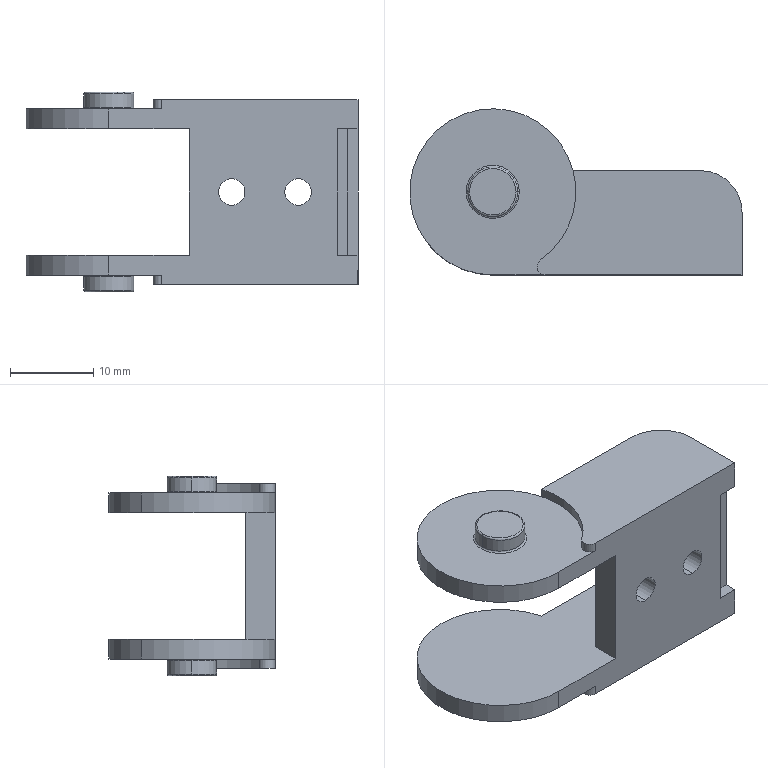Part | STEP file | TWD15-C15-R28-3_fix | 1 solid | 50 faces | box 40 x 20 x 24 mm | volume 4424 mm3 | plane 20 | cylinder 18 | torus 8 | cone 4 | commonest cylinder face diameters 20 x6 3.2 x4 6 x4 2 x2 10 x2
STEP:
#1=CARTESIAN_POINT('',(-15.2,2.5,-1.6));
#2=VERTEX_POINT('',#1);
#3=CARTESIAN_POINT('',(-15.2,2.5,1.6));
#4=VERTEX_POINT('',#3);
#5=CARTESIAN_POINT('',(-15.2,2.5,0.));
#6=DIRECTION('',(0.,-1.,0.));
#7=DIRECTION('',(0.,0.,1.));
#8=AXIS2_PLACEMENT_3D('',#5,#6,#7);
#9=CIRCLE('',#8,1.6);
#10=EDGE_CURVE('',#2,#4,#9,.T.);
#11=ORIENTED_EDGE('',*,*,#10,.F.);
#12=CARTESIAN_POINT('',(-15.2,0.,-1.6));
#13=VERTEX_POINT('',#12);
#14=CARTESIAN_POINT('',(-15.2,0.,-1.6));
#15=DIRECTION('',(0.,-1.,0.));
#16=VECTOR('',#15,1000.);
#17=LINE('',#14,#16);
#18=EDGE_CURVE('',#2,#13,#17,.T.);
#19=ORIENTED_EDGE('',*,*,#18,.T.);
#20=CARTESIAN_POINT('',(-15.2,0.,1.6));
#21=VERTEX_POINT('',#20);
#22=CARTESIAN_POINT('',(-15.2,0.,0.));
#23=DIRECTION('',(0.,-1.,0.));
#24=DIRECTION('',(0.,0.,-1.));
#25=AXIS2_PLACEMENT_3D('',#22,#23,#24);
#26=CIRCLE('',#25,1.6);
#27=EDGE_CURVE('',#13,#21,#26,.T.);
#28=ORIENTED_EDGE('',*,*,#27,.T.);
#29=CARTESIAN_POINT('',(-15.2,0.,1.6));
#30=DIRECTION('',(0.,-1.,0.));
#31=VECTOR('',#30,1000.);
#32=LINE('',#29,#31);
#33=EDGE_CURVE('',#4,#21,#32,.T.);
#34=ORIENTED_EDGE('',*,*,#33,.F.);
#35=EDGE_LOOP('',(#11,#19,#28,#34));
#36=FACE_OUTER_BOUND('',#35,.T.);
#37=CARTESIAN_POINT('',(-15.2,0.,0.));
#38=DIRECTION('',(0.,-1.,0.));
#39=DIRECTION('',(0.000000142,0.,1.));
#40=AXIS2_PLACEMENT_3D('',#37,#38,#39);
#41=CYLINDRICAL_SURFACE('',#40,1.6);
#42=ADVANCED_FACE('',(#36),#41,.F.);
#43=ORIENTED_EDGE('',*,*,#10,.T.);
#44=CARTESIAN_POINT('',(-15.2,3.5,2.6));
#45=VERTEX_POINT('',#44);
#46=CARTESIAN_POINT('',(-15.2,3.5,2.6));
#47=DIRECTION('',(0.,0.7071,0.7071));
#48=VECTOR('',#47,1000.);
#49=LINE('',#46,#48);
#50=EDGE_CURVE('',#4,#45,#49,.T.);
#51=ORIENTED_EDGE('',*,*,#50,.T.);
#52=CARTESIAN_POINT('',(-15.2,3.5,-2.6));
#53=VERTEX_POINT('',#52);
#54=CARTESIAN_POINT('',(-15.2,3.5,0.));
#55=DIRECTION('',(0.,-1.,0.));
#56=DIRECTION('',(0.,0.,1.));
#57=AXIS2_PLACEMENT_3D('',#54,#55,#56);
#58=CIRCLE('',#57,2.6);
#59=EDGE_CURVE('',#53,#45,#58,.T.);
#60=ORIENTED_EDGE('',*,*,#59,.F.);
#61=CARTESIAN_POINT('',(-15.2,3.5,-2.6));
#62=DIRECTION('',(0.,0.7071,-0.7071));
#63=VECTOR('',#62,1000.);
#64=LINE('',#61,#63);
#65=EDGE_CURVE('',#2,#53,#64,.T.);
#66=ORIENTED_EDGE('',*,*,#65,.F.);
#67=EDGE_LOOP('',(#43,#51,#60,#66));
#68=FACE_OUTER_BOUND('',#67,.T.);
#69=CARTESIAN_POINT('',(-15.2,3.5,0.));
#70=DIRECTION('',(0.,1.,0.));
#71=DIRECTION('',(0.,0.,-1.));
#72=AXIS2_PLACEMENT_3D('',#69,#70,#71);
#73=CONICAL_SURFACE('',#72,2.6,0.7854);
#74=ADVANCED_FACE('',(#68),#73,.F.);
#75=CARTESIAN_POINT('',(-7.2,2.5,-1.6));
#76=VERTEX_POINT('',#75);
#77=CARTESIAN_POINT('',(-7.2,2.5,1.6));
#78=VERTEX_POINT('',#77);
#79=CARTESIAN_POINT('',(-7.2,2.5,0.));
#80=DIRECTION('',(0.,-1.,0.));
#81=DIRECTION('',(0.,0.,1.));
#82=AXIS2_PLACEMENT_3D('',#79,#80,#81);
#83=CIRCLE('',#82,1.6);
#84=EDGE_CURVE('',#76,#78,#83,.T.);
#85=ORIENTED_EDGE('',*,*,#84,.F.);
#86=CARTESIAN_POINT('',(-7.2,0.,-1.6));
#87=VERTEX_POINT('',#86);
#88=CARTESIAN_POINT('',(-7.2,0.,-1.6));
#89=DIRECTION('',(0.,-1.,0.));
#90=VECTOR('',#89,1000.);
#91=LINE('',#88,#90);
#92=EDGE_CURVE('',#76,#87,#91,.T.);
#93=ORIENTED_EDGE('',*,*,#92,.T.);
#94=CARTESIAN_POINT('',(-7.2,0.,1.6));
#95=VERTEX_POINT('',#94);
#96=CARTESIAN_POINT('',(-7.2,0.,0.));
#97=DIRECTION('',(0.,-1.,0.));
#98=DIRECTION('',(0.,0.,-1.));
#99=AXIS2_PLACEMENT_3D('',#96,#97,#98);
#100=CIRCLE('',#99,1.6);
#101=EDGE_CURVE('',#87,#95,#100,.T.);
#102=ORIENTED_EDGE('',*,*,#101,.T.);
#103=CARTESIAN_POINT('',(-7.2,0.,1.6));
#104=DIRECTION('',(0.,-1.,0.));
#105=VECTOR('',#104,1000.);
#106=LINE('',#103,#105);
#107=EDGE_CURVE('',#78,#95,#106,.T.);
#108=ORIENTED_EDGE('',*,*,#107,.F.);
#109=EDGE_LOOP('',(#85,#93,#102,#108));
#110=FACE_OUTER_BOUND('',#109,.T.);
#111=CARTESIAN_POINT('',(-7.2,0.,0.));
#112=DIRECTION('',(0.,-1.,0.));
#113=DIRECTION('',(0.000000142,0.,1.));
#114=AXIS2_PLACEMENT_3D('',#111,#112,#113);
#115=CYLINDRICAL_SURFACE('',#114,1.6);
#116=ADVANCED_FACE('',(#110),#115,.F.);
#117=ORIENTED_EDGE('',*,*,#84,.T.);
#118=CARTESIAN_POINT('',(-7.2,3.5,2.6));
#119=VERTEX_POINT('',#118);
#120=CARTESIAN_POINT('',(-7.2,3.5,2.6));
#121=DIRECTION('',(0.,0.7071,0.7071));
#122=VECTOR('',#121,1000.);
#123=LINE('',#120,#122);
#124=EDGE_CURVE('',#78,#119,#123,.T.);
#125=ORIENTED_EDGE('',*,*,#124,.T.);
#126=CARTESIAN_POINT('',(-7.2,3.5,-2.6));
#127=VERTEX_POINT('',#126);
#128=CARTESIAN_POINT('',(-7.2,3.5,0.));
#129=DIRECTION('',(0.,-1.,0.));
#130=DIRECTION('',(-0.000000142,0.,1.));
#131=AXIS2_PLACEMENT_3D('',#128,#129,#130);
#132=CIRCLE('',#131,2.6);
#133=EDGE_CURVE('',#127,#119,#132,.T.);
#134=ORIENTED_EDGE('',*,*,#133,.F.);
#135=CARTESIAN_POINT('',(-7.2,3.5,-2.6));
#136=DIRECTION('',(0.,0.7071,-0.7071));
#137=VECTOR('',#136,1000.);
#138=LINE('',#135,#137);
#139=EDGE_CURVE('',#76,#127,#138,.T.);
#140=ORIENTED_EDGE('',*,*,#139,.F.);
#141=EDGE_LOOP('',(#117,#125,#134,#140));
#142=FACE_OUTER_BOUND('',#141,.T.);
#143=CARTESIAN_POINT('',(-7.2,3.5,0.));
#144=DIRECTION('',(0.,1.,0.));
#145=DIRECTION('',(0.,0.,-1.));
#146=AXIS2_PLACEMENT_3D('',#143,#144,#145);
#147=CONICAL_SURFACE('',#146,2.6,0.7854);
#148=ADVANCED_FACE('',(#142),#147,.F.);
#149=CARTESIAN_POINT('',(-33.2,10.,10.));
#150=VERTEX_POINT('',#149);
#151=CARTESIAN_POINT('',(-26.8,10.,10.));
#152=VERTEX_POINT('',#151);
#153=CARTESIAN_POINT('',(-30.,10.,10.));
#154=DIRECTION('',(0.,0.,-1.));
#155=DIRECTION('',(1.,0.,0.));
#156=AXIS2_PLACEMENT_3D('',#153,#154,#155);
#157=CIRCLE('',#156,3.2);
#158=EDGE_CURVE('',#150,#152,#157,.T.);
#159=ORIENTED_EDGE('',*,*,#158,.F.);
#160=CARTESIAN_POINT('',(-33.,10.,10.2));
#161=VERTEX_POINT('',#160);
#162=CARTESIAN_POINT('',(-33.2,10.,10.2));
#163=DIRECTION('',(0.,-1.,0.));
#164=DIRECTION('',(1.,0.,0.));
#165=AXIS2_PLACEMENT_3D('',#162,#163,#164);
#166=CIRCLE('',#165,0.2);
#167=EDGE_CURVE('',#150,#161,#166,.T.);
#168=ORIENTED_EDGE('',*,*,#167,.T.);
#169=CARTESIAN_POINT('',(-27.,10.,10.2));
#170=VERTEX_POINT('',#169);
#171=CARTESIAN_POINT('',(-30.,10.,10.2));
#172=DIRECTION('',(0.,0.,-1.));
#173=DIRECTION('',(-1.,0.,0.));
#174=AXIS2_PLACEMENT_3D('',#171,#172,#173);
#175=CIRCLE('',#174,3.);
#176=EDGE_CURVE('',#161,#170,#175,.T.);
#177=ORIENTED_EDGE('',*,*,#176,.T.);
#178=CARTESIAN_POINT('',(-26.8,10.,10.2));
#179=DIRECTION('',(0.,1.,0.));
#180=DIRECTION('',(-1.,0.,0.));
#181=AXIS2_PLACEMENT_3D('',#178,#179,#180);
#182=CIRCLE('',#181,0.2);
#183=EDGE_CURVE('',#152,#170,#182,.T.);
#184=ORIENTED_EDGE('',*,*,#183,.F.);
#185=EDGE_LOOP('',(#159,#168,#177,#184));
#186=FACE_OUTER_BOUND('',#185,.T.);
#187=CARTESIAN_POINT('',(-30.,10.,10.2));
#188=DIRECTION('',(0.,0.,-1.));
#189=DIRECTION('',(1.,0.,0.));
#190=AXIS2_PLACEMENT_3D('',#187,#188,#189);
#191=TOROIDAL_SURFACE('',#190,3.2,0.2);
#192=ADVANCED_FACE('',(#186),#191,.F.);
#193=CARTESIAN_POINT('',(-27.,10.,11.8));
#194=VERTEX_POINT('',#193);
#195=CARTESIAN_POINT('',(-33.,10.,11.8));
#196=VERTEX_POINT('',#195);
#197=CARTESIAN_POINT('',(-30.,10.,11.8));
#198=DIRECTION('',(0.,0.,-1.));
#199=DIRECTION('',(-1.,0.,0.));
#200=AXIS2_PLACEMENT_3D('',#197,#198,#199);
#201=CIRCLE('',#200,3.);
#202=EDGE_CURVE('',#194,#196,#201,.T.);
#203=ORIENTED_EDGE('',*,*,#202,.T.);
#204=CARTESIAN_POINT('',(-33.,10.,10.));
#205=DIRECTION('',(0.,0.,-1.));
#206=VECTOR('',#205,1000.);
#207=LINE('',#204,#206);
#208=EDGE_CURVE('',#196,#161,#207,.T.);
#209=ORIENTED_EDGE('',*,*,#208,.T.);
#210=CARTESIAN_POINT('',(-30.,10.,10.2));
#211=DIRECTION('',(0.,0.,-1.));
#212=DIRECTION('',(-1.,0.,0.));
#213=AXIS2_PLACEMENT_3D('',#210,#211,#212);
#214=CIRCLE('',#213,3.);
#215=EDGE_CURVE('',#170,#161,#214,.T.);
#216=ORIENTED_EDGE('',*,*,#215,.F.);
#217=CARTESIAN_POINT('',(-27.,10.,10.));
#218=DIRECTION('',(0.,0.,-1.));
#219=VECTOR('',#218,1000.);
#220=LINE('',#217,#219);
#221=EDGE_CURVE('',#194,#170,#220,.T.);
#222=ORIENTED_EDGE('',*,*,#221,.F.);
#223=EDGE_LOOP('',(#203,#209,#216,#222));
#224=FACE_OUTER_BOUND('',#223,.T.);
#225=CARTESIAN_POINT('',(-30.,10.,10.));
#226=DIRECTION('',(0.,0.,-1.));
#227=DIRECTION('',(1.,0.000000001,0.));
#228=AXIS2_PLACEMENT_3D('',#225,#226,#227);
#229=CYLINDRICAL_SURFACE('',#228,3.);
#230=ADVANCED_FACE('',(#224),#229,.T.);
#231=CARTESIAN_POINT('',(-27.2,10.,12.));
#232=VERTEX_POINT('',#231);
#233=CARTESIAN_POINT('',(-32.8,10.,12.));
#234=VERTEX_POINT('',#233);
#235=CARTESIAN_POINT('',(-30.,10.,12.));
#236=DIRECTION('',(0.,0.,-1.));
#237=DIRECTION('',(-1.,0.,0.));
#238=AXIS2_PLACEMENT_3D('',#235,#236,#237);
#239=CIRCLE('',#238,2.8);
#240=EDGE_CURVE('',#232,#234,#239,.T.);
#241=ORIENTED_EDGE('',*,*,#240,.T.);
#242=CARTESIAN_POINT('',(-32.8,10.,11.8));
#243=DIRECTION('',(0.000000142,-1.,0.));
#244=DIRECTION('',(1.,0.000000142,0.));
#245=AXIS2_PLACEMENT_3D('',#242,#243,#244);
#246=CIRCLE('',#245,0.2);
#247=EDGE_CURVE('',#234,#196,#246,.T.);
#248=ORIENTED_EDGE('',*,*,#247,.T.);
#249=ORIENTED_EDGE('',*,*,#202,.F.);
#250=CARTESIAN_POINT('',(-27.2,10.,11.8));
#251=DIRECTION('',(-0.000000142,1.,0.));
#252=DIRECTION('',(-1.,-0.000000142,0.));
#253=AXIS2_PLACEMENT_3D('',#250,#251,#252);
#254=CIRCLE('',#253,0.2);
#255=EDGE_CURVE('',#232,#194,#254,.T.);
#256=ORIENTED_EDGE('',*,*,#255,.F.);
#257=EDGE_LOOP('',(#241,#248,#249,#256));
#258=FACE_OUTER_BOUND('',#257,.T.);
#259=CARTESIAN_POINT('',(-30.,10.,11.8));
#260=DIRECTION('',(0.,0.,-1.));
#261=DIRECTION('',(1.,0.000000142,0.));
#262=AXIS2_PLACEMENT_3D('',#259,#260,#261);
#263=TOROIDAL_SURFACE('',#262,2.8,0.2);
#264=ADVANCED_FACE('',(#258),#263,.T.);
#265=CARTESIAN_POINT('',(-27.,10.,-11.8));
#266=VERTEX_POINT('',#265);
#267=CARTESIAN_POINT('',(-33.,10.,-11.8));
#268=VERTEX_POINT('',#267);
#269=CARTESIAN_POINT('',(-30.,10.,-11.8));
#270=DIRECTION('',(0.,0.,-1.));
#271=DIRECTION('',(-1.,0.,0.));
#272=AXIS2_PLACEMENT_3D('',#269,#270,#271);
#273=CIRCLE('',#272,3.);
#274=EDGE_CURVE('',#266,#268,#273,.T.);
#275=ORIENTED_EDGE('',*,*,#274,.T.);
#276=CARTESIAN_POINT('',(-32.8,10.,-12.));
#277=VERTEX_POINT('',#276);
#278=CARTESIAN_POINT('',(-32.8,10.,-11.8));
#279=DIRECTION('',(0.,-1.,0.));
#280=DIRECTION('',(1.,0.,0.));
#281=AXIS2_PLACEMENT_3D('',#278,#279,#280);
#282=CIRCLE('',#281,0.2);
#283=EDGE_CURVE('',#268,#277,#282,.T.);
#284=ORIENTED_EDGE('',*,*,#283,.T.);
#285=CARTESIAN_POINT('',(-27.2,10.,-12.));
#286=VERTEX_POINT('',#285);
#287=CARTESIAN_POINT('',(-30.,10.,-12.));
#288=DIRECTION('',(0.,0.,-1.));
#289=DIRECTION('',(1.,-0.000000142,0.));
#290=AXIS2_PLACEMENT_3D('',#287,#288,#289);
#291=CIRCLE('',#290,2.8);
#292=EDGE_CURVE('',#286,#277,#291,.T.);
#293=ORIENTED_EDGE('',*,*,#292,.F.);
#294=CARTESIAN_POINT('',(-27.2,10.,-11.8));
#295=DIRECTION('',(0.,1.,0.));
#296=DIRECTION('',(-1.,0.,0.));
#297=AXIS2_PLACEMENT_3D('',#294,#295,#296);
#298=CIRCLE('',#297,0.2);
#299=EDGE_CURVE('',#266,#286,#298,.T.);
#300=ORIENTED_EDGE('',*,*,#299,.F.);
#301=EDGE_LOOP('',(#275,#284,#293,#300));
#302=FACE_OUTER_BOUND('',#301,.T.);
#303=CARTESIAN_POINT('',(-30.,10.,-11.8));
#304=DIRECTION('',(0.,0.,-1.));
#305=DIRECTION('',(1.,0.,0.));
#306=AXIS2_PLACEMENT_3D('',#303,#304,#305);
#307=TOROIDAL_SURFACE('',#306,2.8,0.2);
#308=ADVANCED_FACE('',(#302),#307,.T.);
#309=CARTESIAN_POINT('',(-27.,10.,-10.2));
#310=VERTEX_POINT('',#309);
#311=CARTESIAN_POINT('',(-33.,10.,-10.2));
#312=VERTEX_POINT('',#311);
#313=CARTESIAN_POINT('',(-30.,10.,-10.2));
#314=DIRECTION('',(0.,0.,-1.));
#315=DIRECTION('',(-1.,0.,0.));
#316=AXIS2_PLACEMENT_3D('',#313,#314,#315);
#317=CIRCLE('',#316,3.);
#318=EDGE_CURVE('',#310,#312,#317,.T.);
#319=ORIENTED_EDGE('',*,*,#318,.T.);
#320=CARTESIAN_POINT('',(-33.,10.,-12.));
#321=DIRECTION('',(0.,0.,-1.));
#322=VECTOR('',#321,1000.);
#323=LINE('',#320,#322);
#324=EDGE_CURVE('',#312,#268,#323,.T.);
#325=ORIENTED_EDGE('',*,*,#324,.T.);
#326=ORIENTED_EDGE('',*,*,#274,.F.);
#327=CARTESIAN_POINT('',(-27.,10.,-12.));
#328=DIRECTION('',(0.,0.,-1.));
#329=VECTOR('',#328,1000.);
#330=LINE('',#327,#329);
#331=EDGE_CURVE('',#310,#266,#330,.T.);
#332=ORIENTED_EDGE('',*,*,#331,.F.);
#333=EDGE_LOOP('',(#319,#325,#326,#332));
#334=FACE_OUTER_BOUND('',#333,.T.);
#335=CARTESIAN_POINT('',(-30.,10.,-12.));
#336=DIRECTION('',(0.,0.,-1.));
#337=DIRECTION('',(1.,0.000000001,0.));
#338=AXIS2_PLACEMENT_3D('',#335,#336,#337);
#339=CYLINDRICAL_SURFACE('',#338,3.);
#340=ADVANCED_FACE('',(#334),#339,.T.);
#341=CARTESIAN_POINT('',(-30.,10.,-10.2));
#342=DIRECTION('',(0.,0.,-1.));
#343=DIRECTION('',(-1.,0.,0.));
#344=AXIS2_PLACEMENT_3D('',#341,#342,#343);
#345=CIRCLE('',#344,3.);
#346=EDGE_CURVE('',#312,#310,#345,.T.);
#347=ORIENTED_EDGE('',*,*,#346,.F.);
#348=CARTESIAN_POINT('',(-33.2,10.,-10.));
#349=VERTEX_POINT('',#348);
#350=CARTESIAN_POINT('',(-33.2,10.,-10.2));
#351=DIRECTION('',(0.000000142,-1.,0.));
#352=DIRECTION('',(1.,0.000000142,0.));
#353=AXIS2_PLACEMENT_3D('',#350,#351,#352);
#354=CIRCLE('',#353,0.2);
#355=EDGE_CURVE('',#312,#349,#354,.T.);
#356=ORIENTED_EDGE('',*,*,#355,.T.);
#357=CARTESIAN_POINT('',(-26.8,10.,-10.));
#358=VERTEX_POINT('',#357);
#359=CARTESIAN_POINT('',(-30.,10.,-10.));
#360=DIRECTION('',(0.,0.,-1.));
#361=DIRECTION('',(-1.,0.,0.));
#362=AXIS2_PLACEMENT_3D('',#359,#360,#361);
#363=CIRCLE('',#362,3.2);
#364=EDGE_CURVE('',#349,#358,#363,.T.);
#365=ORIENTED_EDGE('',*,*,#364,.T.);
#366=CARTESIAN_POINT('',(-26.8,10.,-10.2));
#367=DIRECTION('',(-0.000000142,1.,0.));
#368=DIRECTION('',(-1.,-0.000000142,0.));
#369=AXIS2_PLACEMENT_3D('',#366,#367,#368);
#370=CIRCLE('',#369,0.2);
#371=EDGE_CURVE('',#310,#358,#370,.T.);
#372=ORIENTED_EDGE('',*,*,#371,.F.);
#373=EDGE_LOOP('',(#347,#356,#365,#372));
#374=FACE_OUTER_BOUND('',#373,.T.);
#375=CARTESIAN_POINT('',(-30.,10.,-10.2));
#376=DIRECTION('',(0.,0.,-1.));
#377=DIRECTION('',(1.,0.000000142,0.));
#378=AXIS2_PLACEMENT_3D('',#375,#376,#377);
#379=TOROIDAL_SURFACE('',#378,3.2,0.2);
#380=ADVANCED_FACE('',(#374),#379,.F.);
#381=CARTESIAN_POINT('',(-37.925,16.099,-7.6));
#382=VERTEX_POINT('',#381);
#383=CARTESIAN_POINT('',(-30.,0.,-7.6));
#384=VERTEX_POINT('',#383);
#385=CARTESIAN_POINT('',(-30.,10.,-7.6));
#386=DIRECTION('',(0.,0.,1.));
#387=DIRECTION('',(0.,-1.,0.));
#388=AXIS2_PLACEMENT_3D('',#385,#386,#387);
#389=CIRCLE('',#388,10.);
#390=EDGE_CURVE('',#382,#384,#389,.T.);
#391=ORIENTED_EDGE('',*,*,#390,.F.);
#392=CARTESIAN_POINT('',(-37.925,16.099,-10.));
#393=VERTEX_POINT('',#392);
#394=CARTESIAN_POINT('',(-37.925,16.099,11.1));
#395=DIRECTION('',(0.,0.,-1.));
#396=VECTOR('',#395,1000.);
#397=LINE('',#394,#396);
#398=EDGE_CURVE('',#382,#393,#397,.T.);
#399=ORIENTED_EDGE('',*,*,#398,.T.);
#400=CARTESIAN_POINT('',(-30.,0.,-10.));
#401=VERTEX_POINT('',#400);
#402=CARTESIAN_POINT('',(-30.,10.,-10.));
#403=DIRECTION('',(0.,0.,1.));
#404=DIRECTION('',(0.9667,0.256,0.));
#405=AXIS2_PLACEMENT_3D('',#402,#403,#404);
#406=CIRCLE('',#405,10.);
#407=EDGE_CURVE('',#393,#401,#406,.T.);
#408=ORIENTED_EDGE('',*,*,#407,.T.);
#409=CARTESIAN_POINT('',(-30.,0.,-7.6));
#410=DIRECTION('',(0.,0.,-1.));
#411=VECTOR('',#410,1000.);
#412=LINE('',#409,#411);
#413=EDGE_CURVE('',#384,#401,#412,.T.);
#414=ORIENTED_EDGE('',*,*,#413,.F.);
#415=EDGE_LOOP('',(#391,#399,#408,#414));
#416=FACE_OUTER_BOUND('',#415,.T.);
#417=CARTESIAN_POINT('',(-30.,10.,11.1));
#418=DIRECTION('',(0.,0.,-1.));
#419=DIRECTION('',(-0.7925,0.6099,0.));
#420=AXIS2_PLACEMENT_3D('',#417,#418,#419);
#421=CYLINDRICAL_SURFACE('',#420,10.);
#422=ADVANCED_FACE('',(#416),#421,.T.);
#423=CARTESIAN_POINT('',(-37.925,16.099,10.));
#424=VERTEX_POINT('',#423);
#425=CARTESIAN_POINT('',(-30.,0.,10.));
#426=VERTEX_POINT('',#425);
#427=CARTESIAN_POINT('',(-30.,10.,10.));
#428=DIRECTION('',(0.,0.,1.));
#429=DIRECTION('',(0.,-1.,0.));
#430=AXIS2_PLACEMENT_3D('',#427,#428,#429);
#431=CIRCLE('',#430,10.);
#432=EDGE_CURVE('',#424,#426,#431,.T.);
#433=ORIENTED_EDGE('',*,*,#432,.F.);
#434=CARTESIAN_POINT('',(-37.925,16.099,7.6));
#435=VERTEX_POINT('',#434);
#436=CARTESIAN_POINT('',(-37.925,16.099,11.1));
#437=DIRECTION('',(0.,0.,-1.));
#438=VECTOR('',#437,1000.);
#439=LINE('',#436,#438);
#440=EDGE_CURVE('',#424,#435,#439,.T.);
#441=ORIENTED_EDGE('',*,*,#440,.T.);
#442=CARTESIAN_POINT('',(-30.,0.,7.6));
#443=VERTEX_POINT('',#442);
#444=CARTESIAN_POINT('',(-30.,10.,7.6));
#445=DIRECTION('',(0.,0.,1.));
#446=DIRECTION('',(0.9667,0.256,0.));
#447=AXIS2_PLACEMENT_3D('',#444,#445,#446);
#448=CIRCLE('',#447,10.);
#449=EDGE_CURVE('',#435,#443,#448,.T.);
#450=ORIENTED_EDGE('',*,*,#449,.T.);
#451=CARTESIAN_POINT('',(-30.,0.,10.));
#452=DIRECTION('',(0.,0.,-1.));
#453=VECTOR('',#452,1000.);
#454=LINE('',#451,#453);
#455=EDGE_CURVE('',#426,#443,#454,.T.);
#456=ORIENTED_EDGE('',*,*,#455,.F.);
#457=EDGE_LOOP('',(#433,#441,#450,#456));
#458=FACE_OUTER_BOUND('',#457,.T.);
#459=CARTESIAN_POINT('',(-30.,10.,11.1));
#460=DIRECTION('',(0.,0.,-1.));
#461=DIRECTION('',(-0.7925,0.6099,0.));
#462=AXIS2_PLACEMENT_3D('',#459,#460,#461);
#463=CYLINDRICAL_SURFACE('',#462,10.);
#464=ADVANCED_FACE('',(#458),#463,.T.);
#465=CARTESIAN_POINT('',(-23.675,0.,-11.1));
#466=VERTEX_POINT('',#465);
#467=CARTESIAN_POINT('',(-23.675,0.,-10.));
#468=VERTEX_POINT('',#467);
#469=CARTESIAN_POINT('',(-23.675,0.,-10.));
#470=DIRECTION('',(0.,0.,1.));
#471=VECTOR('',#470,1000.);
#472=LINE('',#469,#471);
#473=EDGE_CURVE('',#466,#468,#472,.T.);
#474=ORIENTED_EDGE('',*,*,#473,.F.);
#475=CARTESIAN_POINT('',(0.,0.,-11.1));
#476=VERTEX_POINT('',#475);
#477=CARTESIAN_POINT('',(-23.675,0.,-11.1));
#478=DIRECTION('',(1.,0.,0.));
#479=VECTOR('',#478,1000.);
#480=LINE('',#477,#479);
#481=EDGE_CURVE('',#466,#476,#480,.T.);
#482=ORIENTED_EDGE('',*,*,#481,.T.);
#483=CARTESIAN_POINT('',(0.,0.,-7.6));
#484=VERTEX_POINT('',#483);
#485=CARTESIAN_POINT('',(0.,0.,-11.1));
#486=DIRECTION('',(0.,0.,-1.));
#487=VECTOR('',#486,1000.);
#488=LINE('',#485,#487);
#489=EDGE_CURVE('',#484,#476,#488,.T.);
#490=ORIENTED_EDGE('',*,*,#489,.F.);
#491=CARTESIAN_POINT('',(-2.5,0.,-7.6));
#492=VERTEX_POINT('',#491);
#493=CARTESIAN_POINT('',(0.,0.,-7.6));
#494=DIRECTION('',(1.,0.,0.));
#495=VECTOR('',#494,1000.);
#496=LINE('',#493,#495);
#497=EDGE_CURVE('',#492,#484,#496,.T.);
#498=ORIENTED_EDGE('',*,*,#497,.F.);
#499=CARTESIAN_POINT('',(-2.5,0.,7.6));
#500=VERTEX_POINT('',#499);
#501=CARTESIAN_POINT('',(-2.5,0.,-7.6));
#502=DIRECTION('',(0.,0.,-1.));
#503=VECTOR('',#502,1000.);
#504=LINE('',#501,#503);
#505=EDGE_CURVE('',#500,#492,#504,.T.);
#506=ORIENTED_EDGE('',*,*,#505,.F.);
#507=CARTESIAN_POINT('',(0.,0.,7.6));
#508=VERTEX_POINT('',#507);
#509=CARTESIAN_POINT('',(-2.5,0.,7.6));
#510=DIRECTION('',(1.,0.,0.));
#511=VECTOR('',#510,1000.);
#512=LINE('',#509,#511);
#513=EDGE_CURVE('',#500,#508,#512,.T.);
#514=ORIENTED_EDGE('',*,*,#513,.T.);
#515=CARTESIAN_POINT('',(0.,0.,11.1));
#516=VERTEX_POINT('',#515);
#517=CARTESIAN_POINT('',(0.,0.,7.6));
#518=DIRECTION('',(0.,0.,-1.));
#519=VECTOR('',#518,1000.);
#520=LINE('',#517,#519);
#521=EDGE_CURVE('',#516,#508,#520,.T.);
#522=ORIENTED_EDGE('',*,*,#521,.F.);
#523=CARTESIAN_POINT('',(-23.675,0.,11.1));
#524=VERTEX_POINT('',#523);
#525=CARTESIAN_POINT('',(0.,0.,11.1));
#526=DIRECTION('',(1.,0.,0.));
#527=VECTOR('',#526,1000.);
#528=LINE('',#525,#527);
#529=EDGE_CURVE('',#524,#516,#528,.T.);
#530=ORIENTED_EDGE('',*,*,#529,.F.);
#531=CARTESIAN_POINT('',(-23.675,0.,10.));
#532=VERTEX_POINT('',#531);
#533=CARTESIAN_POINT('',(-23.675,0.,11.1));
#534=DIRECTION('',(0.,0.,-1.));
#535=VECTOR('',#534,1000.);
#536=LINE('',#533,#535);
#537=EDGE_CURVE('',#524,#532,#536,.T.);
#538=ORIENTED_EDGE('',*,*,#537,.T.);
#539=CARTESIAN_POINT('',(-23.675,0.,10.));
#540=DIRECTION('',(1.,0.,0.));
#541=VECTOR('',#540,1000.);
#542=LINE('',#539,#541);
#543=EDGE_CURVE('',#426,#532,#542,.T.);
#544=ORIENTED_EDGE('',*,*,#543,.F.);
#545=ORIENTED_EDGE('',*,*,#455,.T.);
#546=CARTESIAN_POINT('',(-20.32,0.,7.6));
#547=VERTEX_POINT('',#546);
#548=CARTESIAN_POINT('',(-30.,0.,7.6));
#549=DIRECTION('',(1.,0.,0.));
#550=VECTOR('',#549,1000.);
#551=LINE('',#548,#550);
#552=EDGE_CURVE('',#443,#547,#551,.T.);
#553=ORIENTED_EDGE('',*,*,#552,.T.);
#554=CARTESIAN_POINT('',(-20.32,0.,-7.6));
#555=VERTEX_POINT('',#554);
#556=CARTESIAN_POINT('',(-20.32,0.,7.6));
#557=DIRECTION('',(0.,0.,-1.));
#558=VECTOR('',#557,1000.);
#559=LINE('',#556,#558);
#560=EDGE_CURVE('',#547,#555,#559,.T.);
#561=ORIENTED_EDGE('',*,*,#560,.T.);
#562=CARTESIAN_POINT('',(-20.32,0.,-7.6));
#563=DIRECTION('',(1.,0.,0.));
#564=VECTOR('',#563,1000.);
#565=LINE('',#562,#564);
#566=EDGE_CURVE('',#384,#555,#565,.T.);
#567=ORIENTED_EDGE('',*,*,#566,.F.);
#568=ORIENTED_EDGE('',*,*,#413,.T.);
#569=CARTESIAN_POINT('',(-30.,0.,-10.));
#570=DIRECTION('',(1.,0.,0.));
#571=VECTOR('',#570,1000.);
#572=LINE('',#569,#571);
#573=EDGE_CURVE('',#401,#468,#572,.T.);
#574=ORIENTED_EDGE('',*,*,#573,.T.);
#575=EDGE_LOOP('',(#474,#482,#490,#498,#506,#514,#522,#530,#538,#544,#545,#553,#561,#567,#568,#574));
#576=FACE_OUTER_BOUND('',#575,.T.);
#577=CARTESIAN_POINT('',(-7.2,0.,0.));
#578=DIRECTION('',(0.,-1.,0.));
#579=DIRECTION('',(0.,0.,-1.));
#580=AXIS2_PLACEMENT_3D('',#577,#578,#579);
#581=CIRCLE('',#580,1.6);
#582=EDGE_CURVE('',#95,#87,#581,.T.);
#583=ORIENTED_EDGE('',*,*,#582,.F.);
#584=ORIENTED_EDGE('',*,*,#101,.F.);
#585=EDGE_LOOP('',(#583,#584));
#586=FACE_BOUND('',#585,.T.);
#587=CARTESIAN_POINT('',(-15.2,0.,0.));
#588=DIRECTION('',(0.,-1.,0.));
#589=DIRECTION('',(0.,0.,-1.));
#590=AXIS2_PLACEMENT_3D('',#587,#588,#589);
#591=CIRCLE('',#590,1.6);
#592=EDGE_CURVE('',#21,#13,#591,.T.);
#593=ORIENTED_EDGE('',*,*,#592,.F.);
#594=ORIENTED_EDGE('',*,*,#27,.F.);
#595=EDGE_LOOP('',(#593,#594));
#596=FACE_BOUND('',#595,.T.);
#597=CARTESIAN_POINT('',(-30.,0.,-11.1));
#598=DIRECTION('',(0.,-1.,0.));
#599=DIRECTION('',(1.,0.,0.));
#600=AXIS2_PLACEMENT_3D('',#597,#598,#599);
#601=PLANE('',#600);
#602=ADVANCED_FACE('',(#576,#586,#596),#601,.T.);
#603=CARTESIAN_POINT('',(-24.25,1.818,-11.1));
#604=VERTEX_POINT('',#603);
#605=CARTESIAN_POINT('',(-23.675,1.,-11.1));
#606=DIRECTION('',(0.,0.,1.));
#607=DIRECTION('',(0.,-1.,0.));
#608=AXIS2_PLACEMENT_3D('',#605,#606,#607);
#609=CIRCLE('',#608,1.);
#610=EDGE_CURVE('',#604,#466,#609,.T.);
#611=ORIENTED_EDGE('',*,*,#610,.F.);
#612=CARTESIAN_POINT('',(-20.333,12.56,-11.1));
#613=VERTEX_POINT('',#612);
#614=CARTESIAN_POINT('',(-30.,10.,-11.1));
#615=DIRECTION('',(0.,0.,1.));
#616=DIRECTION('',(0.575,-0.8182,0.));
#617=AXIS2_PLACEMENT_3D('',#614,#615,#616);
#618=CIRCLE('',#617,10.);
#619=EDGE_CURVE('',#604,#613,#618,.T.);
#620=ORIENTED_EDGE('',*,*,#619,.T.);
#621=CARTESIAN_POINT('',(-5.,12.56,-11.1));
#622=VERTEX_POINT('',#621);
#623=CARTESIAN_POINT('',(-20.333,12.56,-11.1));
#624=DIRECTION('',(-1.,0.,0.));
#625=VECTOR('',#624,1000.);
#626=LINE('',#623,#625);
#627=EDGE_CURVE('',#622,#613,#626,.T.);
#628=ORIENTED_EDGE('',*,*,#627,.F.);
#629=CARTESIAN_POINT('',(0.,7.56,-11.1));
#630=VERTEX_POINT('',#629);
#631=CARTESIAN_POINT('',(-5.,7.56,-11.1));
#632=DIRECTION('',(0.,0.,1.));
#633=DIRECTION('',(0.,1.,0.));
#634=AXIS2_PLACEMENT_3D('',#631,#632,#633);
#635=CIRCLE('',#634,5.);
#636=EDGE_CURVE('',#630,#622,#635,.T.);
#637=ORIENTED_EDGE('',*,*,#636,.F.);
#638=CARTESIAN_POINT('',(0.,7.56,-11.1));
#639=DIRECTION('',(0.,1.,0.));
#640=VECTOR('',#639,1000.);
#641=LINE('',#638,#640);
#642=EDGE_CURVE('',#476,#630,#641,.T.);
#643=ORIENTED_EDGE('',*,*,#642,.F.);
#644=ORIENTED_EDGE('',*,*,#481,.F.);
#645=EDGE_LOOP('',(#611,#620,#628,#637,#643,#644));
#646=FACE_OUTER_BOUND('',#645,.T.);
#647=CARTESIAN_POINT('',(-24.704,0.,-11.1));
#648=DIRECTION('',(0.,0.,-1.));
#649=DIRECTION('',(0.,1.,0.));
#650=AXIS2_PLACEMENT_3D('',#647,#648,#649);
#651=PLANE('',#650);
#652=ADVANCED_FACE('',(#646),#651,.T.);
#653=ORIENTED_EDGE('',*,*,#440,.F.);
#654=CARTESIAN_POINT('',(-20.333,12.56,10.));
#655=VERTEX_POINT('',#654);
#656=CARTESIAN_POINT('',(-30.,10.,10.));
#657=DIRECTION('',(0.,0.,1.));
#658=DIRECTION('',(0.,-1.,0.));
#659=AXIS2_PLACEMENT_3D('',#656,#657,#658);
#660=CIRCLE('',#659,10.);
#661=EDGE_CURVE('',#655,#424,#660,.T.);
#662=ORIENTED_EDGE('',*,*,#661,.F.);
#663=CARTESIAN_POINT('',(-20.333,12.56,7.6));
#664=VERTEX_POINT('',#663);
#665=CARTESIAN_POINT('',(-20.333,12.56,10.));
#666=DIRECTION('',(0.,0.,-1.));
#667=VECTOR('',#666,1000.);
#668=LINE('',#665,#667);
#669=EDGE_CURVE('',#655,#664,#668,.T.);
#670=ORIENTED_EDGE('',*,*,#669,.T.);
#671=CARTESIAN_POINT('',(-30.,10.,7.6));
#672=DIRECTION('',(0.,0.,1.));
#673=DIRECTION('',(0.9667,0.256,0.));
#674=AXIS2_PLACEMENT_3D('',#671,#672,#673);
#675=CIRCLE('',#674,10.);
#676=EDGE_CURVE('',#664,#435,#675,.T.);
#677=ORIENTED_EDGE('',*,*,#676,.T.);
#678=EDGE_LOOP('',(#653,#662,#670,#677));
#679=FACE_OUTER_BOUND('',#678,.T.);
#680=CARTESIAN_POINT('',(-30.,10.,11.1));
#681=DIRECTION('',(0.,0.,-1.));
#682=DIRECTION('',(-0.7925,0.6099,0.));
#683=AXIS2_PLACEMENT_3D('',#680,#681,#682);
#684=CYLINDRICAL_SURFACE('',#683,10.);
#685=ADVANCED_FACE('',(#679),#684,.T.);
#686=CARTESIAN_POINT('',(-24.25,1.818,11.1));
#687=VERTEX_POINT('',#686);
#688=CARTESIAN_POINT('',(-23.675,1.,11.1));
#689=DIRECTION('',(0.,0.,-1.));
#690=DIRECTION('',(-0.575,0.8182,0.));
#691=AXIS2_PLACEMENT_3D('',#688,#689,#690);
#692=CIRCLE('',#691,1.);
#693=EDGE_CURVE('',#524,#687,#692,.T.);
#694=ORIENTED_EDGE('',*,*,#693,.F.);
#695=ORIENTED_EDGE('',*,*,#529,.T.);
#696=CARTESIAN_POINT('',(0.,7.56,11.1));
#697=VERTEX_POINT('',#696);
#698=CARTESIAN_POINT('',(0.,0.,11.1));
#699=DIRECTION('',(0.,1.,0.));
#700=VECTOR('',#699,1000.);
#701=LINE('',#698,#700);
#702=EDGE_CURVE('',#516,#697,#701,.T.);
#703=ORIENTED_EDGE('',*,*,#702,.T.);
#704=CARTESIAN_POINT('',(-5.,12.56,11.1));
#705=VERTEX_POINT('',#704);
#706=CARTESIAN_POINT('',(-5.,7.56,11.1));
#707=DIRECTION('',(0.,0.,1.));
#708=DIRECTION('',(1.,0.,0.));
#709=AXIS2_PLACEMENT_3D('',#706,#707,#708);
#710=CIRCLE('',#709,5.);
#711=EDGE_CURVE('',#697,#705,#710,.T.);
#712=ORIENTED_EDGE('',*,*,#711,.T.);
#713=CARTESIAN_POINT('',(-20.333,12.56,11.1));
#714=VERTEX_POINT('',#713);
#715=CARTESIAN_POINT('',(-5.,12.56,11.1));
#716=DIRECTION('',(-1.,0.,0.));
#717=VECTOR('',#716,1000.);
#718=LINE('',#715,#717);
#719=EDGE_CURVE('',#705,#714,#718,.T.);
#720=ORIENTED_EDGE('',*,*,#719,.T.);
#721=CARTESIAN_POINT('',(-30.,10.,11.1));
#722=DIRECTION('',(0.,0.,-1.));
#723=DIRECTION('',(0.9667,0.256,0.));
#724=AXIS2_PLACEMENT_3D('',#721,#722,#723);
#725=CIRCLE('',#724,10.);
#726=EDGE_CURVE('',#714,#687,#725,.T.);
#727=ORIENTED_EDGE('',*,*,#726,.T.);
#728=EDGE_LOOP('',(#694,#695,#703,#712,#720,#727));
#729=FACE_OUTER_BOUND('',#728,.T.);
#730=CARTESIAN_POINT('',(-24.696,0.,11.1));
#731=DIRECTION('',(0.,0.,1.));
#732=DIRECTION('',(1.,0.,0.));
#733=AXIS2_PLACEMENT_3D('',#730,#731,#732);
#734=PLANE('',#733);
#735=ADVANCED_FACE('',(#729),#734,.T.);
#736=CARTESIAN_POINT('',(-5.,12.56,-7.6));
#737=VERTEX_POINT('',#736);
#738=CARTESIAN_POINT('',(-20.333,12.56,-7.6));
#739=VERTEX_POINT('',#738);
#740=CARTESIAN_POINT('',(-20.333,12.56,-7.6));
#741=DIRECTION('',(-1.,0.,0.));
#742=VECTOR('',#741,1000.);
#743=LINE('',#740,#742);
#744=EDGE_CURVE('',#737,#739,#743,.T.);
#745=ORIENTED_EDGE('',*,*,#744,.F.);
#746=CARTESIAN_POINT('',(-5.,12.56,-7.6));
#747=DIRECTION('',(0.,0.,-1.));
#748=VECTOR('',#747,1000.);
#749=LINE('',#746,#748);
#750=EDGE_CURVE('',#737,#622,#749,.T.);
#751=ORIENTED_EDGE('',*,*,#750,.T.);
#752=ORIENTED_EDGE('',*,*,#627,.T.);
#753=CARTESIAN_POINT('',(-20.333,12.56,-10.));
#754=VERTEX_POINT('',#753);
#755=CARTESIAN_POINT('',(-20.333,12.56,-11.1));
#756=DIRECTION('',(0.,0.,1.));
#757=VECTOR('',#756,1000.);
#758=LINE('',#755,#757);
#759=EDGE_CURVE('',#613,#754,#758,.T.);
#760=ORIENTED_EDGE('',*,*,#759,.T.);
#761=CARTESIAN_POINT('',(-20.333,12.56,-10.));
#762=DIRECTION('',(0.,0.,-1.));
#763=VECTOR('',#762,1000.);
#764=LINE('',#761,#763);
#765=EDGE_CURVE('',#739,#754,#764,.T.);
#766=ORIENTED_EDGE('',*,*,#765,.F.);
#767=EDGE_LOOP('',(#745,#751,#752,#760,#766));
#768=FACE_OUTER_BOUND('',#767,.T.);
#769=CARTESIAN_POINT('',(-20.333,12.56,-7.6));
#770=DIRECTION('',(0.,1.,0.));
#771=DIRECTION('',(1.,0.,0.));
#772=AXIS2_PLACEMENT_3D('',#769,#770,#771);
#773=PLANE('',#772);
#774=ADVANCED_FACE('',(#768),#773,.T.);
#775=ORIENTED_EDGE('',*,*,#398,.F.);
#776=CARTESIAN_POINT('',(-30.,10.,-7.6));
#777=DIRECTION('',(0.,0.,1.));
#778=DIRECTION('',(0.,-1.,0.));
#779=AXIS2_PLACEMENT_3D('',#776,#777,#778);
#780=CIRCLE('',#779,10.);
#781=EDGE_CURVE('',#739,#382,#780,.T.);
#782=ORIENTED_EDGE('',*,*,#781,.F.);
#783=ORIENTED_EDGE('',*,*,#765,.T.);
#784=CARTESIAN_POINT('',(-30.,10.,-10.));
#785=DIRECTION('',(0.,0.,1.));
#786=DIRECTION('',(0.9667,0.256,0.));
#787=AXIS2_PLACEMENT_3D('',#784,#785,#786);
#788=CIRCLE('',#787,10.);
#789=EDGE_CURVE('',#754,#393,#788,.T.);
#790=ORIENTED_EDGE('',*,*,#789,.T.);
#791=EDGE_LOOP('',(#775,#782,#783,#790));
#792=FACE_OUTER_BOUND('',#791,.T.);
#793=CARTESIAN_POINT('',(-30.,10.,11.1));
#794=DIRECTION('',(0.,0.,-1.));
#795=DIRECTION('',(-0.7925,0.6099,0.));
#796=AXIS2_PLACEMENT_3D('',#793,#794,#795);
#797=CYLINDRICAL_SURFACE('',#796,10.);
#798=ADVANCED_FACE('',(#792),#797,.T.);
#799=CARTESIAN_POINT('',(0.,7.56,-7.6));
#800=VERTEX_POINT('',#799);
#801=CARTESIAN_POINT('',(-5.,7.56,-7.6));
#802=DIRECTION('',(0.,0.,1.));
#803=DIRECTION('',(0.,1.,0.));
#804=AXIS2_PLACEMENT_3D('',#801,#802,#803);
#805=CIRCLE('',#804,5.);
#806=EDGE_CURVE('',#800,#737,#805,.T.);
#807=ORIENTED_EDGE('',*,*,#806,.F.);
#808=CARTESIAN_POINT('',(0.,7.56,-7.6));
#809=DIRECTION('',(0.,0.,-1.));
#810=VECTOR('',#809,1000.);
#811=LINE('',#808,#810);
#812=EDGE_CURVE('',#800,#630,#811,.T.);
#813=ORIENTED_EDGE('',*,*,#812,.T.);
#814=ORIENTED_EDGE('',*,*,#636,.T.);
#815=ORIENTED_EDGE('',*,*,#750,.F.);
#816=EDGE_LOOP('',(#807,#813,#814,#815));
#817=FACE_OUTER_BOUND('',#816,.T.);
#818=CARTESIAN_POINT('',(-5.,7.56,11.1));
#819=DIRECTION('',(0.,0.,-1.));
#820=DIRECTION('',(0.,1.,0.));
#821=AXIS2_PLACEMENT_3D('',#818,#819,#820);
#822=CYLINDRICAL_SURFACE('',#821,5.);
#823=ADVANCED_FACE('',(#817),#822,.T.);
#824=CARTESIAN_POINT('',(-5.,12.56,7.6));
#825=VERTEX_POINT('',#824);
#826=CARTESIAN_POINT('',(-5.,12.56,11.1));
#827=DIRECTION('',(0.,0.,-1.));
#828=VECTOR('',#827,1000.);
#829=LINE('',#826,#828);
#830=EDGE_CURVE('',#705,#825,#829,.T.);
#831=ORIENTED_EDGE('',*,*,#830,.T.);
#832=CARTESIAN_POINT('',(-5.,12.56,7.6));
#833=DIRECTION('',(-1.,0.,0.));
#834=VECTOR('',#833,1000.);
#835=LINE('',#832,#834);
#836=EDGE_CURVE('',#825,#664,#835,.T.);
#837=ORIENTED_EDGE('',*,*,#836,.T.);
#838=ORIENTED_EDGE('',*,*,#669,.F.);
#839=CARTESIAN_POINT('',(-20.333,12.56,10.));
#840=DIRECTION('',(0.,0.,-1.));
#841=VECTOR('',#840,1000.);
#842=LINE('',#839,#841);
#843=EDGE_CURVE('',#714,#655,#842,.T.);
#844=ORIENTED_EDGE('',*,*,#843,.F.);
#845=ORIENTED_EDGE('',*,*,#719,.F.);
#846=EDGE_LOOP('',(#831,#837,#838,#844,#845));
#847=FACE_OUTER_BOUND('',#846,.T.);
#848=CARTESIAN_POINT('',(-20.333,12.56,11.1));
#849=DIRECTION('',(0.,1.,0.));
#850=DIRECTION('',(1.,0.,0.));
#851=AXIS2_PLACEMENT_3D('',#848,#849,#850);
#852=PLANE('',#851);
#853=ADVANCED_FACE('',(#847),#852,.T.);
#854=ORIENTED_EDGE('',*,*,#521,.T.);
#855=CARTESIAN_POINT('',(0.,1.5,7.6));
#856=VERTEX_POINT('',#855);
#857=CARTESIAN_POINT('',(0.,0.,7.6));
#858=DIRECTION('',(0.,1.,0.));
#859=VECTOR('',#858,1000.);
#860=LINE('',#857,#859);
#861=EDGE_CURVE('',#508,#856,#860,.T.);
#862=ORIENTED_EDGE('',*,*,#861,.T.);
#863=CARTESIAN_POINT('',(0.,1.5,-7.6));
#864=VERTEX_POINT('',#863);
#865=CARTESIAN_POINT('',(0.,1.5,7.6));
#866=DIRECTION('',(0.,0.,-1.));
#867=VECTOR('',#866,1000.);
#868=LINE('',#865,#867);
#869=EDGE_CURVE('',#856,#864,#868,.T.);
#870=ORIENTED_EDGE('',*,*,#869,.T.);
#871=CARTESIAN_POINT('',(0.,1.5,-7.6));
#872=DIRECTION('',(0.,1.,0.));
#873=VECTOR('',#872,1000.);
#874=LINE('',#871,#873);
#875=EDGE_CURVE('',#484,#864,#874,.T.);
#876=ORIENTED_EDGE('',*,*,#875,.F.);
#877=ORIENTED_EDGE('',*,*,#489,.T.);
#878=ORIENTED_EDGE('',*,*,#642,.T.);
#879=ORIENTED_EDGE('',*,*,#812,.F.);
#880=CARTESIAN_POINT('',(0.,3.5,-7.6));
#881=VERTEX_POINT('',#880);
#882=CARTESIAN_POINT('',(0.,7.56,-7.6));
#883=DIRECTION('',(0.,1.,0.));
#884=VECTOR('',#883,1000.);
#885=LINE('',#882,#884);
#886=EDGE_CURVE('',#881,#800,#885,.T.);
#887=ORIENTED_EDGE('',*,*,#886,.F.);
#888=CARTESIAN_POINT('',(0.,3.5,7.6));
#889=VERTEX_POINT('',#888);
#890=CARTESIAN_POINT('',(0.,3.5,-7.6));
#891=DIRECTION('',(0.,0.,-1.));
#892=VECTOR('',#891,1000.);
#893=LINE('',#890,#892);
#894=EDGE_CURVE('',#889,#881,#893,.T.);
#895=ORIENTED_EDGE('',*,*,#894,.F.);
#896=CARTESIAN_POINT('',(0.,7.56,7.6));
#897=VERTEX_POINT('',#896);
#898=CARTESIAN_POINT('',(0.,3.5,7.6));
#899=DIRECTION('',(0.,1.,0.));
#900=VECTOR('',#899,1000.);
#901=LINE('',#898,#900);
#902=EDGE_CURVE('',#889,#897,#901,.T.);
#903=ORIENTED_EDGE('',*,*,#902,.T.);
#904=CARTESIAN_POINT('',(0.,7.56,7.6));
#905=DIRECTION('',(0.,0.,-1.));
#906=VECTOR('',#905,1000.);
#907=LINE('',#904,#906);
#908=EDGE_CURVE('',#697,#897,#907,.T.);
#909=ORIENTED_EDGE('',*,*,#908,.F.);
#910=ORIENTED_EDGE('',*,*,#702,.F.);
#911=EDGE_LOOP('',(#854,#862,#870,#876,#877,#878,#879,#887,#895,#903,#909,#910));
#912=FACE_OUTER_BOUND('',#911,.T.);
#913=CARTESIAN_POINT('',(0.,0.,-11.1));
#914=DIRECTION('',(1.,0.,0.));
#915=DIRECTION('',(0.,1.,0.));
#916=AXIS2_PLACEMENT_3D('',#913,#914,#915);
#917=PLANE('',#916);
#918=ADVANCED_FACE('',(#912),#917,.T.);
#919=ORIENTED_EDGE('',*,*,#908,.T.);
#920=CARTESIAN_POINT('',(-5.,7.56,7.6));
#921=DIRECTION('',(0.,0.,1.));
#922=DIRECTION('',(1.,0.,0.));
#923=AXIS2_PLACEMENT_3D('',#920,#921,#922);
#924=CIRCLE('',#923,5.);
#925=EDGE_CURVE('',#897,#825,#924,.T.);
#926=ORIENTED_EDGE('',*,*,#925,.T.);
#927=ORIENTED_EDGE('',*,*,#830,.F.);
#928=ORIENTED_EDGE('',*,*,#711,.F.);
#929=EDGE_LOOP('',(#919,#926,#927,#928));
#930=FACE_OUTER_BOUND('',#929,.T.);
#931=CARTESIAN_POINT('',(-5.,7.56,11.1));
#932=DIRECTION('',(0.,0.,-1.));
#933=DIRECTION('',(0.,1.,0.));
#934=AXIS2_PLACEMENT_3D('',#931,#932,#933);
#935=CYLINDRICAL_SURFACE('',#934,5.);
#936=ADVANCED_FACE('',(#930),#935,.T.);
#937=ORIENTED_EDGE('',*,*,#676,.F.);
#938=ORIENTED_EDGE('',*,*,#836,.F.);
#939=ORIENTED_EDGE('',*,*,#925,.F.);
#940=ORIENTED_EDGE('',*,*,#902,.F.);
#941=CARTESIAN_POINT('',(-20.32,3.5,7.6));
#942=VERTEX_POINT('',#941);
#943=CARTESIAN_POINT('',(0.,3.5,7.6));
#944=DIRECTION('',(-1.,0.,0.));
#945=VECTOR('',#944,1000.);
#946=LINE('',#943,#945);
#947=EDGE_CURVE('',#889,#942,#946,.T.);
#948=ORIENTED_EDGE('',*,*,#947,.T.);
#949=CARTESIAN_POINT('',(-20.32,3.5,7.6));
#950=DIRECTION('',(0.,-1.,0.));
#951=VECTOR('',#950,1000.);
#952=LINE('',#949,#951);
#953=EDGE_CURVE('',#942,#547,#952,.T.);
#954=ORIENTED_EDGE('',*,*,#953,.T.);
#955=ORIENTED_EDGE('',*,*,#552,.F.);
#956=ORIENTED_EDGE('',*,*,#449,.F.);
#957=EDGE_LOOP('',(#937,#938,#939,#940,#948,#954,#955,#956));
#958=FACE_OUTER_BOUND('',#957,.T.);
#959=CARTESIAN_POINT('',(-40.964,-0.000000011,7.6));
#960=DIRECTION('',(0.,0.,-1.));
#961=DIRECTION('',(0.,1.,0.));
#962=AXIS2_PLACEMENT_3D('',#959,#960,#961);
#963=PLANE('',#962);
#964=ADVANCED_FACE('',(#958),#963,.T.);
#965=ORIENTED_EDGE('',*,*,#781,.T.);
#966=ORIENTED_EDGE('',*,*,#390,.T.);
#967=ORIENTED_EDGE('',*,*,#566,.T.);
#968=CARTESIAN_POINT('',(-20.32,3.5,-7.6));
#969=VERTEX_POINT('',#968);
#970=CARTESIAN_POINT('',(-20.32,0.,-7.6));
#971=DIRECTION('',(0.,-1.,0.));
#972=VECTOR('',#971,1000.);
#973=LINE('',#970,#972);
#974=EDGE_CURVE('',#969,#555,#973,.T.);
#975=ORIENTED_EDGE('',*,*,#974,.F.);
#976=CARTESIAN_POINT('',(-20.32,3.5,-7.6));
#977=DIRECTION('',(-1.,0.,0.));
#978=VECTOR('',#977,1000.);
#979=LINE('',#976,#978);
#980=EDGE_CURVE('',#881,#969,#979,.T.);
#981=ORIENTED_EDGE('',*,*,#980,.F.);
#982=ORIENTED_EDGE('',*,*,#886,.T.);
#983=ORIENTED_EDGE('',*,*,#806,.T.);
#984=ORIENTED_EDGE('',*,*,#744,.T.);
#985=EDGE_LOOP('',(#965,#966,#967,#975,#981,#982,#983,#984));
#986=FACE_OUTER_BOUND('',#985,.T.);
#987=CARTESIAN_POINT('',(-40.786,-0.000005598,-7.6));
#988=DIRECTION('',(0.,0.,1.));
#989=DIRECTION('',(1.,0.,0.));
#990=AXIS2_PLACEMENT_3D('',#987,#988,#989);
#991=PLANE('',#990);
#992=ADVANCED_FACE('',(#986),#991,.T.);
#993=ORIENTED_EDGE('',*,*,#980,.T.);
#994=CARTESIAN_POINT('',(-20.32,3.5,-7.6));
#995=DIRECTION('',(0.,0.,-1.));
#996=VECTOR('',#995,1000.);
#997=LINE('',#994,#996);
#998=EDGE_CURVE('',#942,#969,#997,.T.);
#999=ORIENTED_EDGE('',*,*,#998,.F.);
#1000=ORIENTED_EDGE('',*,*,#947,.F.);
#1001=ORIENTED_EDGE('',*,*,#894,.T.);
#1002=EDGE_LOOP('',(#993,#999,#1000,#1001));
#1003=FACE_OUTER_BOUND('',#1002,.T.);
#1004=ORIENTED_EDGE('',*,*,#133,.T.);
#1005=CARTESIAN_POINT('',(-7.2,3.5,0.));
#1006=DIRECTION('',(0.,-1.,0.));
#1007=DIRECTION('',(-0.000000142,0.,1.));
#1008=AXIS2_PLACEMENT_3D('',#1005,#1006,#1007);
#1009=CIRCLE('',#1008,2.6);
#1010=EDGE_CURVE('',#119,#127,#1009,.T.);
#1011=ORIENTED_EDGE('',*,*,#1010,.T.);
#1012=EDGE_LOOP('',(#1004,#1011));
#1013=FACE_BOUND('',#1012,.T.);
#1014=ORIENTED_EDGE('',*,*,#59,.T.);
#1015=CARTESIAN_POINT('',(-15.2,3.5,0.));
#1016=DIRECTION('',(0.,-1.,0.));
#1017=DIRECTION('',(0.,0.,1.));
#1018=AXIS2_PLACEMENT_3D('',#1015,#1016,#1017);
#1019=CIRCLE('',#1018,2.6);
#1020=EDGE_CURVE('',#45,#53,#1019,.T.);
#1021=ORIENTED_EDGE('',*,*,#1020,.T.);
#1022=EDGE_LOOP('',(#1014,#1021));
#1023=FACE_BOUND('',#1022,.T.);
#1024=CARTESIAN_POINT('',(-20.32,3.5,7.6));
#1025=DIRECTION('',(0.,1.,0.));
#1026=DIRECTION('',(1.,0.,0.));
#1027=AXIS2_PLACEMENT_3D('',#1024,#1025,#1026);
#1028=PLANE('',#1027);
#1029=ADVANCED_FACE('',(#1003,#1013,#1023),#1028,.T.);
#1030=ORIENTED_EDGE('',*,*,#974,.T.);
#1031=ORIENTED_EDGE('',*,*,#560,.F.);
#1032=ORIENTED_EDGE('',*,*,#953,.F.);
#1033=ORIENTED_EDGE('',*,*,#998,.T.);
#1034=EDGE_LOOP('',(#1030,#1031,#1032,#1033));
#1035=FACE_OUTER_BOUND('',#1034,.T.);
#1036=CARTESIAN_POINT('',(-20.32,0.,7.6));
#1037=DIRECTION('',(-1.,0.,0.));
#1038=DIRECTION('',(0.,1.,0.));
#1039=AXIS2_PLACEMENT_3D('',#1036,#1037,#1038);
#1040=PLANE('',#1039);
#1041=ADVANCED_FACE('',(#1035),#1040,.T.);
#1042=CARTESIAN_POINT('',(-2.5,2.5,7.6));
#1043=VERTEX_POINT('',#1042);
#1044=CARTESIAN_POINT('',(-2.5,0.,7.6));
#1045=DIRECTION('',(0.,1.,0.));
#1046=VECTOR('',#1045,1000.);
#1047=LINE('',#1044,#1046);
#1048=EDGE_CURVE('',#500,#1043,#1047,.T.);
#1049=ORIENTED_EDGE('',*,*,#1048,.T.);
#1050=CARTESIAN_POINT('',(-1.25,2.5,7.6));
#1051=VERTEX_POINT('',#1050);
#1052=CARTESIAN_POINT('',(-2.5,2.5,7.6));
#1053=DIRECTION('',(1.,0.,0.));
#1054=VECTOR('',#1053,1000.);
#1055=LINE('',#1052,#1054);
#1056=EDGE_CURVE('',#1043,#1051,#1055,.T.);
#1057=ORIENTED_EDGE('',*,*,#1056,.T.);
#1058=CARTESIAN_POINT('',(-1.25,1.5,7.6));
#1059=VERTEX_POINT('',#1058);
#1060=CARTESIAN_POINT('',(-1.25,2.5,7.6));
#1061=DIRECTION('',(0.,-1.,0.));
#1062=VECTOR('',#1061,1000.);
#1063=LINE('',#1060,#1062);
#1064=EDGE_CURVE('',#1051,#1059,#1063,.T.);
#1065=ORIENTED_EDGE('',*,*,#1064,.T.);
#1066=CARTESIAN_POINT('',(-1.25,1.5,7.6));
#1067=DIRECTION('',(1.,0.,0.));
#1068=VECTOR('',#1067,1000.);
#1069=LINE('',#1066,#1068);
#1070=EDGE_CURVE('',#1059,#856,#1069,.T.);
#1071=ORIENTED_EDGE('',*,*,#1070,.T.);
#1072=ORIENTED_EDGE('',*,*,#861,.F.);
#1073=ORIENTED_EDGE('',*,*,#513,.F.);
#1074=EDGE_LOOP('',(#1049,#1057,#1065,#1071,#1072,#1073));
#1075=FACE_OUTER_BOUND('',#1074,.T.);
#1076=CARTESIAN_POINT('',(-2.5,0.,7.6));
#1077=DIRECTION('',(0.,0.,-1.));
#1078=DIRECTION('',(0.,1.,0.));
#1079=AXIS2_PLACEMENT_3D('',#1076,#1077,#1078);
#1080=PLANE('',#1079);
#1081=ADVANCED_FACE('',(#1075),#1080,.T.);
#1082=ORIENTED_EDGE('',*,*,#497,.T.);
#1083=ORIENTED_EDGE('',*,*,#875,.T.);
#1084=CARTESIAN_POINT('',(-1.25,1.5,-7.6));
#1085=VERTEX_POINT('',#1084);
#1086=CARTESIAN_POINT('',(0.,1.5,-7.6));
#1087=DIRECTION('',(1.,0.,0.));
#1088=VECTOR('',#1087,1000.);
#1089=LINE('',#1086,#1088);
#1090=EDGE_CURVE('',#1085,#864,#1089,.T.);
#1091=ORIENTED_EDGE('',*,*,#1090,.F.);
#1092=CARTESIAN_POINT('',(-1.25,2.5,-7.6));
#1093=VERTEX_POINT('',#1092);
#1094=CARTESIAN_POINT('',(-1.25,1.5,-7.6));
#1095=DIRECTION('',(0.,-1.,0.));
#1096=VECTOR('',#1095,1000.);
#1097=LINE('',#1094,#1096);
#1098=EDGE_CURVE('',#1093,#1085,#1097,.T.);
#1099=ORIENTED_EDGE('',*,*,#1098,.F.);
#1100=CARTESIAN_POINT('',(-2.5,2.5,-7.6));
#1101=VERTEX_POINT('',#1100);
#1102=CARTESIAN_POINT('',(-1.25,2.5,-7.6));
#1103=DIRECTION('',(1.,0.,0.));
#1104=VECTOR('',#1103,1000.);
#1105=LINE('',#1102,#1104);
#1106=EDGE_CURVE('',#1101,#1093,#1105,.T.);
#1107=ORIENTED_EDGE('',*,*,#1106,.F.);
#1108=CARTESIAN_POINT('',(-2.5,2.5,-7.6));
#1109=DIRECTION('',(0.,1.,0.));
#1110=VECTOR('',#1109,1000.);
#1111=LINE('',#1108,#1110);
#1112=EDGE_CURVE('',#492,#1101,#1111,.T.);
#1113=ORIENTED_EDGE('',*,*,#1112,.F.);
#1114=EDGE_LOOP('',(#1082,#1083,#1091,#1099,#1107,#1113));
#1115=FACE_OUTER_BOUND('',#1114,.T.);
#1116=CARTESIAN_POINT('',(-2.5,0.,-7.6));
#1117=DIRECTION('',(0.,0.,1.));
#1118=DIRECTION('',(1.,0.,0.));
#1119=AXIS2_PLACEMENT_3D('',#1116,#1117,#1118);
#1120=PLANE('',#1119);
#1121=ADVANCED_FACE('',(#1115),#1120,.T.);
#1122=ORIENTED_EDGE('',*,*,#1090,.T.);
#1123=ORIENTED_EDGE('',*,*,#869,.F.);
#1124=ORIENTED_EDGE('',*,*,#1070,.F.);
#1125=CARTESIAN_POINT('',(-1.25,1.5,7.6));
#1126=DIRECTION('',(0.,0.,-1.));
#1127=VECTOR('',#1126,1000.);
#1128=LINE('',#1125,#1127);
#1129=EDGE_CURVE('',#1059,#1085,#1128,.T.);
#1130=ORIENTED_EDGE('',*,*,#1129,.T.);
#1131=EDGE_LOOP('',(#1122,#1123,#1124,#1130));
#1132=FACE_OUTER_BOUND('',#1131,.T.);
#1133=CARTESIAN_POINT('',(-1.25,1.5,-7.6));
#1134=DIRECTION('',(0.,-1.,0.));
#1135=DIRECTION('',(1.,0.,0.));
#1136=AXIS2_PLACEMENT_3D('',#1133,#1134,#1135);
#1137=PLANE('',#1136);
#1138=ADVANCED_FACE('',(#1132),#1137,.T.);
#1139=ORIENTED_EDGE('',*,*,#1098,.T.);
#1140=ORIENTED_EDGE('',*,*,#1129,.F.);
#1141=ORIENTED_EDGE('',*,*,#1064,.F.);
#1142=CARTESIAN_POINT('',(-1.25,2.5,7.6));
#1143=DIRECTION('',(0.,0.,-1.));
#1144=VECTOR('',#1143,1000.);
#1145=LINE('',#1142,#1144);
#1146=EDGE_CURVE('',#1051,#1093,#1145,.T.);
#1147=ORIENTED_EDGE('',*,*,#1146,.T.);
#1148=EDGE_LOOP('',(#1139,#1140,#1141,#1147));
#1149=FACE_OUTER_BOUND('',#1148,.T.);
#1150=CARTESIAN_POINT('',(-1.25,1.5,7.6));
#1151=DIRECTION('',(-1.,0.,0.));
#1152=DIRECTION('',(0.,1.,0.));
#1153=AXIS2_PLACEMENT_3D('',#1150,#1151,#1152);
#1154=PLANE('',#1153);
#1155=ADVANCED_FACE('',(#1149),#1154,.T.);
#1156=ORIENTED_EDGE('',*,*,#1106,.T.);
#1157=ORIENTED_EDGE('',*,*,#1146,.F.);
#1158=ORIENTED_EDGE('',*,*,#1056,.F.);
#1159=CARTESIAN_POINT('',(-2.5,2.5,7.6));
#1160=DIRECTION('',(0.,0.,-1.));
#1161=VECTOR('',#1160,1000.);
#1162=LINE('',#1159,#1161);
#1163=EDGE_CURVE('',#1043,#1101,#1162,.T.);
#1164=ORIENTED_EDGE('',*,*,#1163,.T.);
#1165=EDGE_LOOP('',(#1156,#1157,#1158,#1164));
#1166=FACE_OUTER_BOUND('',#1165,.T.);
#1167=CARTESIAN_POINT('',(-2.5,2.5,-7.6));
#1168=DIRECTION('',(0.,-1.,0.));
#1169=DIRECTION('',(1.,0.,0.));
#1170=AXIS2_PLACEMENT_3D('',#1167,#1168,#1169);
#1171=PLANE('',#1170);
#1172=ADVANCED_FACE('',(#1166),#1171,.T.);
#1173=ORIENTED_EDGE('',*,*,#1112,.T.);
#1174=ORIENTED_EDGE('',*,*,#1163,.F.);
#1175=ORIENTED_EDGE('',*,*,#1048,.F.);
#1176=ORIENTED_EDGE('',*,*,#505,.T.);
#1177=EDGE_LOOP('',(#1173,#1174,#1175,#1176));
#1178=FACE_OUTER_BOUND('',#1177,.T.);
#1179=CARTESIAN_POINT('',(-2.5,0.,-7.6));
#1180=DIRECTION('',(1.,0.,0.));
#1181=DIRECTION('',(0.,1.,0.));
#1182=AXIS2_PLACEMENT_3D('',#1179,#1180,#1181);
#1183=PLANE('',#1182);
#1184=ADVANCED_FACE('',(#1178),#1183,.T.);
#1185=ORIENTED_EDGE('',*,*,#843,.T.);
#1186=CARTESIAN_POINT('',(-24.25,1.818,10.));
#1187=VERTEX_POINT('',#1186);
#1188=CARTESIAN_POINT('',(-30.,10.,10.));
#1189=DIRECTION('',(0.,0.,1.));
#1190=DIRECTION('',(0.9667,0.256,0.));
#1191=AXIS2_PLACEMENT_3D('',#1188,#1189,#1190);
#1192=CIRCLE('',#1191,10.);
#1193=EDGE_CURVE('',#1187,#655,#1192,.T.);
#1194=ORIENTED_EDGE('',*,*,#1193,.F.);
#1195=CARTESIAN_POINT('',(-24.25,1.818,10.));
#1196=DIRECTION('',(0.,0.,-1.));
#1197=VECTOR('',#1196,1000.);
#1198=LINE('',#1195,#1197);
#1199=EDGE_CURVE('',#687,#1187,#1198,.T.);
#1200=ORIENTED_EDGE('',*,*,#1199,.F.);
#1201=ORIENTED_EDGE('',*,*,#726,.F.);
#1202=EDGE_LOOP('',(#1185,#1194,#1200,#1201));
#1203=FACE_OUTER_BOUND('',#1202,.T.);
#1204=CARTESIAN_POINT('',(-30.,10.,11.8));
#1205=DIRECTION('',(0.,0.,-1.));
#1206=DIRECTION('',(0.9667,0.256,0.));
#1207=AXIS2_PLACEMENT_3D('',#1204,#1205,#1206);
#1208=CYLINDRICAL_SURFACE('',#1207,10.);
#1209=ADVANCED_FACE('',(#1203),#1208,.F.);
#1210=ORIENTED_EDGE('',*,*,#693,.T.);
#1211=ORIENTED_EDGE('',*,*,#1199,.T.);
#1212=CARTESIAN_POINT('',(-23.675,1.,10.));
#1213=DIRECTION('',(0.,0.,1.));
#1214=DIRECTION('',(-0.575,0.8182,0.));
#1215=AXIS2_PLACEMENT_3D('',#1212,#1213,#1214);
#1216=CIRCLE('',#1215,1.);
#1217=EDGE_CURVE('',#1187,#532,#1216,.T.);
#1218=ORIENTED_EDGE('',*,*,#1217,.T.);
#1219=ORIENTED_EDGE('',*,*,#537,.F.);
#1220=EDGE_LOOP('',(#1210,#1211,#1218,#1219));
#1221=FACE_OUTER_BOUND('',#1220,.T.);
#1222=CARTESIAN_POINT('',(-23.675,1.,11.8));
#1223=DIRECTION('',(0.,0.,-1.));
#1224=DIRECTION('',(0.,-1.,0.));
#1225=AXIS2_PLACEMENT_3D('',#1222,#1223,#1224);
#1226=CYLINDRICAL_SURFACE('',#1225,1.);
#1227=ADVANCED_FACE('',(#1221),#1226,.T.);
#1228=ORIENTED_EDGE('',*,*,#1217,.F.);
#1229=ORIENTED_EDGE('',*,*,#1193,.T.);
#1230=ORIENTED_EDGE('',*,*,#661,.T.);
#1231=ORIENTED_EDGE('',*,*,#432,.T.);
#1232=ORIENTED_EDGE('',*,*,#543,.T.);
#1233=EDGE_LOOP('',(#1228,#1229,#1230,#1231,#1232));
#1234=FACE_OUTER_BOUND('',#1233,.T.);
#1235=CARTESIAN_POINT('',(-30.,10.,10.));
#1236=DIRECTION('',(0.,0.,-1.));
#1237=DIRECTION('',(1.,0.,0.));
#1238=AXIS2_PLACEMENT_3D('',#1235,#1236,#1237);
#1239=CIRCLE('',#1238,3.2);
#1240=EDGE_CURVE('',#152,#150,#1239,.T.);
#1241=ORIENTED_EDGE('',*,*,#1240,.T.);
#1242=ORIENTED_EDGE('',*,*,#158,.T.);
#1243=EDGE_LOOP('',(#1241,#1242));
#1244=FACE_BOUND('',#1243,.T.);
#1245=CARTESIAN_POINT('',(-40.273,-0.0000247,10.));
#1246=DIRECTION('',(0.,0.,1.));
#1247=DIRECTION('',(1.,0.,0.));
#1248=AXIS2_PLACEMENT_3D('',#1245,#1246,#1247);
#1249=PLANE('',#1248);
#1250=ADVANCED_FACE('',(#1234,#1244),#1249,.T.);
#1251=ORIENTED_EDGE('',*,*,#610,.T.);
#1252=ORIENTED_EDGE('',*,*,#473,.T.);
#1253=CARTESIAN_POINT('',(-24.25,1.818,-10.));
#1254=VERTEX_POINT('',#1253);
#1255=CARTESIAN_POINT('',(-23.675,1.,-10.));
#1256=DIRECTION('',(0.,0.,1.));
#1257=DIRECTION('',(0.,-1.,0.));
#1258=AXIS2_PLACEMENT_3D('',#1255,#1256,#1257);
#1259=CIRCLE('',#1258,1.);
#1260=EDGE_CURVE('',#1254,#468,#1259,.T.);
#1261=ORIENTED_EDGE('',*,*,#1260,.F.);
#1262=CARTESIAN_POINT('',(-24.25,1.818,-10.));
#1263=DIRECTION('',(0.,0.,1.));
#1264=VECTOR('',#1263,1000.);
#1265=LINE('',#1262,#1264);
#1266=EDGE_CURVE('',#604,#1254,#1265,.T.);
#1267=ORIENTED_EDGE('',*,*,#1266,.F.);
#1268=EDGE_LOOP('',(#1251,#1252,#1261,#1267));
#1269=FACE_OUTER_BOUND('',#1268,.T.);
#1270=CARTESIAN_POINT('',(-23.675,1.,-11.8));
#1271=DIRECTION('',(0.,0.,1.));
#1272=DIRECTION('',(-0.575,0.8182,0.));
#1273=AXIS2_PLACEMENT_3D('',#1270,#1271,#1272);
#1274=CYLINDRICAL_SURFACE('',#1273,1.);
#1275=ADVANCED_FACE('',(#1269),#1274,.T.);
#1276=ORIENTED_EDGE('',*,*,#619,.F.);
#1277=ORIENTED_EDGE('',*,*,#1266,.T.);
#1278=CARTESIAN_POINT('',(-30.,10.,-10.));
#1279=DIRECTION('',(0.,0.,1.));
#1280=DIRECTION('',(0.575,-0.8182,0.));
#1281=AXIS2_PLACEMENT_3D('',#1278,#1279,#1280);
#1282=CIRCLE('',#1281,10.);
#1283=EDGE_CURVE('',#1254,#754,#1282,.T.);
#1284=ORIENTED_EDGE('',*,*,#1283,.T.);
#1285=ORIENTED_EDGE('',*,*,#759,.F.);
#1286=EDGE_LOOP('',(#1276,#1277,#1284,#1285));
#1287=FACE_OUTER_BOUND('',#1286,.T.);
#1288=CARTESIAN_POINT('',(-30.,10.,-11.8));
#1289=DIRECTION('',(0.,0.,1.));
#1290=DIRECTION('',(0.575,-0.8182,0.));
#1291=AXIS2_PLACEMENT_3D('',#1288,#1289,#1290);
#1292=CYLINDRICAL_SURFACE('',#1291,10.);
#1293=ADVANCED_FACE('',(#1287),#1292,.F.);
#1294=ORIENTED_EDGE('',*,*,#1260,.T.);
#1295=ORIENTED_EDGE('',*,*,#573,.F.);
#1296=ORIENTED_EDGE('',*,*,#407,.F.);
#1297=ORIENTED_EDGE('',*,*,#789,.F.);
#1298=ORIENTED_EDGE('',*,*,#1283,.F.);
#1299=EDGE_LOOP('',(#1294,#1295,#1296,#1297,#1298));
#1300=FACE_OUTER_BOUND('',#1299,.T.);
#1301=CARTESIAN_POINT('',(-30.,10.,-10.));
#1302=DIRECTION('',(0.,0.,-1.));
#1303=DIRECTION('',(-1.,0.,0.));
#1304=AXIS2_PLACEMENT_3D('',#1301,#1302,#1303);
#1305=CIRCLE('',#1304,3.2);
#1306=EDGE_CURVE('',#358,#349,#1305,.T.);
#1307=ORIENTED_EDGE('',*,*,#1306,.F.);
#1308=ORIENTED_EDGE('',*,*,#364,.F.);
#1309=EDGE_LOOP('',(#1307,#1308));
#1310=FACE_BOUND('',#1309,.T.);
#1311=CARTESIAN_POINT('',(-40.097,-0.00002436,-10.));
#1312=DIRECTION('',(0.,0.,-1.));
#1313=DIRECTION('',(0.,1.,0.));
#1314=AXIS2_PLACEMENT_3D('',#1311,#1312,#1313);
#1315=PLANE('',#1314);
#1316=ADVANCED_FACE('',(#1300,#1310),#1315,.T.);
#1317=ORIENTED_EDGE('',*,*,#292,.T.);
#1318=CARTESIAN_POINT('',(-30.,10.,-12.));
#1319=DIRECTION('',(0.,0.,-1.));
#1320=DIRECTION('',(1.,-0.000000142,0.));
#1321=AXIS2_PLACEMENT_3D('',#1318,#1319,#1320);
#1322=CIRCLE('',#1321,2.8);
#1323=EDGE_CURVE('',#277,#286,#1322,.T.);
#1324=ORIENTED_EDGE('',*,*,#1323,.T.);
#1325=EDGE_LOOP('',(#1317,#1324));
#1326=FACE_OUTER_BOUND('',#1325,.T.);
#1327=CARTESIAN_POINT('',(-32.8,7.2,-12.));
#1328=DIRECTION('',(0.,0.,-1.));
#1329=DIRECTION('',(0.,1.,0.));
#1330=AXIS2_PLACEMENT_3D('',#1327,#1328,#1329);
#1331=PLANE('',#1330);
#1332=ADVANCED_FACE('',(#1326),#1331,.T.);
#1333=ORIENTED_EDGE('',*,*,#240,.F.);
#1334=CARTESIAN_POINT('',(-30.,10.,12.));
#1335=DIRECTION('',(0.,0.,-1.));
#1336=DIRECTION('',(-1.,0.,0.));
#1337=AXIS2_PLACEMENT_3D('',#1334,#1335,#1336);
#1338=CIRCLE('',#1337,2.8);
#1339=EDGE_CURVE('',#234,#232,#1338,.T.);
#1340=ORIENTED_EDGE('',*,*,#1339,.F.);
#1341=EDGE_LOOP('',(#1333,#1340));
#1342=FACE_OUTER_BOUND('',#1341,.T.);
#1343=CARTESIAN_POINT('',(-27.2,7.2,12.));
#1344=DIRECTION('',(0.,0.,1.));
#1345=DIRECTION('',(0.,1.,0.));
#1346=AXIS2_PLACEMENT_3D('',#1343,#1344,#1345);
#1347=PLANE('',#1346);
#1348=ADVANCED_FACE('',(#1342),#1347,.T.);
#1349=ORIENTED_EDGE('',*,*,#355,.F.);
#1350=ORIENTED_EDGE('',*,*,#318,.F.);
#1351=ORIENTED_EDGE('',*,*,#371,.T.);
#1352=ORIENTED_EDGE('',*,*,#1306,.T.);
#1353=EDGE_LOOP('',(#1349,#1350,#1351,#1352));
#1354=FACE_OUTER_BOUND('',#1353,.T.);
#1355=CARTESIAN_POINT('',(-30.,10.,-10.2));
#1356=DIRECTION('',(0.,0.,-1.));
#1357=DIRECTION('',(1.,0.000000142,0.));
#1358=AXIS2_PLACEMENT_3D('',#1355,#1356,#1357);
#1359=TOROIDAL_SURFACE('',#1358,3.2,0.2);
#1360=ADVANCED_FACE('',(#1354),#1359,.F.);
#1361=ORIENTED_EDGE('',*,*,#324,.F.);
#1362=ORIENTED_EDGE('',*,*,#346,.T.);
#1363=ORIENTED_EDGE('',*,*,#331,.T.);
#1364=CARTESIAN_POINT('',(-30.,10.,-11.8));
#1365=DIRECTION('',(0.,0.,-1.));
#1366=DIRECTION('',(-1.,0.,0.));
#1367=AXIS2_PLACEMENT_3D('',#1364,#1365,#1366);
#1368=CIRCLE('',#1367,3.);
#1369=EDGE_CURVE('',#268,#266,#1368,.T.);
#1370=ORIENTED_EDGE('',*,*,#1369,.F.);
#1371=EDGE_LOOP('',(#1361,#1362,#1363,#1370));
#1372=FACE_OUTER_BOUND('',#1371,.T.);
#1373=CARTESIAN_POINT('',(-30.,10.,-12.));
#1374=DIRECTION('',(0.,0.,-1.));
#1375=DIRECTION('',(1.,0.000000001,0.));
#1376=AXIS2_PLACEMENT_3D('',#1373,#1374,#1375);
#1377=CYLINDRICAL_SURFACE('',#1376,3.);
#1378=ADVANCED_FACE('',(#1372),#1377,.T.);
#1379=ORIENTED_EDGE('',*,*,#283,.F.);
#1380=ORIENTED_EDGE('',*,*,#1369,.T.);
#1381=ORIENTED_EDGE('',*,*,#299,.T.);
#1382=ORIENTED_EDGE('',*,*,#1323,.F.);
#1383=EDGE_LOOP('',(#1379,#1380,#1381,#1382));
#1384=FACE_OUTER_BOUND('',#1383,.T.);
#1385=CARTESIAN_POINT('',(-30.,10.,-11.8));
#1386=DIRECTION('',(0.,0.,-1.));
#1387=DIRECTION('',(1.,0.,0.));
#1388=AXIS2_PLACEMENT_3D('',#1385,#1386,#1387);
#1389=TOROIDAL_SURFACE('',#1388,2.8,0.2);
#1390=ADVANCED_FACE('',(#1384),#1389,.T.);
#1391=ORIENTED_EDGE('',*,*,#247,.F.);
#1392=ORIENTED_EDGE('',*,*,#1339,.T.);
#1393=ORIENTED_EDGE('',*,*,#255,.T.);
#1394=CARTESIAN_POINT('',(-30.,10.,11.8));
#1395=DIRECTION('',(0.,0.,-1.));
#1396=DIRECTION('',(-1.,0.,0.));
#1397=AXIS2_PLACEMENT_3D('',#1394,#1395,#1396);
#1398=CIRCLE('',#1397,3.);
#1399=EDGE_CURVE('',#196,#194,#1398,.T.);
#1400=ORIENTED_EDGE('',*,*,#1399,.F.);
#1401=EDGE_LOOP('',(#1391,#1392,#1393,#1400));
#1402=FACE_OUTER_BOUND('',#1401,.T.);
#1403=CARTESIAN_POINT('',(-30.,10.,11.8));
#1404=DIRECTION('',(0.,0.,-1.));
#1405=DIRECTION('',(1.,0.000000142,0.));
#1406=AXIS2_PLACEMENT_3D('',#1403,#1404,#1405);
#1407=TOROIDAL_SURFACE('',#1406,2.8,0.2);
#1408=ADVANCED_FACE('',(#1402),#1407,.T.);
#1409=ORIENTED_EDGE('',*,*,#208,.F.);
#1410=ORIENTED_EDGE('',*,*,#1399,.T.);
#1411=ORIENTED_EDGE('',*,*,#221,.T.);
#1412=ORIENTED_EDGE('',*,*,#176,.F.);
#1413=EDGE_LOOP('',(#1409,#1410,#1411,#1412));
#1414=FACE_OUTER_BOUND('',#1413,.T.);
#1415=CARTESIAN_POINT('',(-30.,10.,10.));
#1416=DIRECTION('',(0.,0.,-1.));
#1417=DIRECTION('',(1.,0.000000001,0.));
#1418=AXIS2_PLACEMENT_3D('',#1415,#1416,#1417);
#1419=CYLINDRICAL_SURFACE('',#1418,3.);
#1420=ADVANCED_FACE('',(#1414),#1419,.T.);
#1421=ORIENTED_EDGE('',*,*,#167,.F.);
#1422=ORIENTED_EDGE('',*,*,#1240,.F.);
#1423=ORIENTED_EDGE('',*,*,#183,.T.);
#1424=ORIENTED_EDGE('',*,*,#215,.T.);
#1425=EDGE_LOOP('',(#1421,#1422,#1423,#1424));
#1426=FACE_OUTER_BOUND('',#1425,.T.);
#1427=CARTESIAN_POINT('',(-30.,10.,10.2));
#1428=DIRECTION('',(0.,0.,-1.));
#1429=DIRECTION('',(1.,0.,0.));
#1430=AXIS2_PLACEMENT_3D('',#1427,#1428,#1429);
#1431=TOROIDAL_SURFACE('',#1430,3.2,0.2);
#1432=ADVANCED_FACE('',(#1426),#1431,.F.);
#1433=ORIENTED_EDGE('',*,*,#124,.F.);
#1434=CARTESIAN_POINT('',(-7.2,2.5,0.));
#1435=DIRECTION('',(0.,-1.,0.));
#1436=DIRECTION('',(0.,0.,1.));
#1437=AXIS2_PLACEMENT_3D('',#1434,#1435,#1436);
#1438=CIRCLE('',#1437,1.6);
#1439=EDGE_CURVE('',#78,#76,#1438,.T.);
#1440=ORIENTED_EDGE('',*,*,#1439,.T.);
#1441=ORIENTED_EDGE('',*,*,#139,.T.);
#1442=ORIENTED_EDGE('',*,*,#1010,.F.);
#1443=EDGE_LOOP('',(#1433,#1440,#1441,#1442));
#1444=FACE_OUTER_BOUND('',#1443,.T.);
#1445=CARTESIAN_POINT('',(-7.2,3.5,0.));
#1446=DIRECTION('',(0.,1.,0.));
#1447=DIRECTION('',(0.,0.,-1.));
#1448=AXIS2_PLACEMENT_3D('',#1445,#1446,#1447);
#1449=CONICAL_SURFACE('',#1448,2.6,0.7854);
#1450=ADVANCED_FACE('',(#1444),#1449,.F.);
#1451=ORIENTED_EDGE('',*,*,#92,.F.);
#1452=ORIENTED_EDGE('',*,*,#1439,.F.);
#1453=ORIENTED_EDGE('',*,*,#107,.T.);
#1454=ORIENTED_EDGE('',*,*,#582,.T.);
#1455=EDGE_LOOP('',(#1451,#1452,#1453,#1454));
#1456=FACE_OUTER_BOUND('',#1455,.T.);
#1457=CARTESIAN_POINT('',(-7.2,0.,0.));
#1458=DIRECTION('',(0.,-1.,0.));
#1459=DIRECTION('',(0.000000142,0.,1.));
#1460=AXIS2_PLACEMENT_3D('',#1457,#1458,#1459);
#1461=CYLINDRICAL_SURFACE('',#1460,1.6);
#1462=ADVANCED_FACE('',(#1456),#1461,.F.);
#1463=ORIENTED_EDGE('',*,*,#50,.F.);
#1464=CARTESIAN_POINT('',(-15.2,2.5,0.));
#1465=DIRECTION('',(0.,-1.,0.));
#1466=DIRECTION('',(0.,0.,1.));
#1467=AXIS2_PLACEMENT_3D('',#1464,#1465,#1466);
#1468=CIRCLE('',#1467,1.6);
#1469=EDGE_CURVE('',#4,#2,#1468,.T.);
#1470=ORIENTED_EDGE('',*,*,#1469,.T.);
#1471=ORIENTED_EDGE('',*,*,#65,.T.);
#1472=ORIENTED_EDGE('',*,*,#1020,.F.);
#1473=EDGE_LOOP('',(#1463,#1470,#1471,#1472));
#1474=FACE_OUTER_BOUND('',#1473,.T.);
#1475=CARTESIAN_POINT('',(-15.2,3.5,0.));
#1476=DIRECTION('',(0.,1.,0.));
#1477=DIRECTION('',(0.,0.,-1.));
#1478=AXIS2_PLACEMENT_3D('',#1475,#1476,#1477);
#1479=CONICAL_SURFACE('',#1478,2.6,0.7854);
#1480=ADVANCED_FACE('',(#1474),#1479,.F.);
#1481=ORIENTED_EDGE('',*,*,#18,.F.);
#1482=ORIENTED_EDGE('',*,*,#1469,.F.);
#1483=ORIENTED_EDGE('',*,*,#33,.T.);
#1484=ORIENTED_EDGE('',*,*,#592,.T.);
#1485=EDGE_LOOP('',(#1481,#1482,#1483,#1484));
#1486=FACE_OUTER_BOUND('',#1485,.T.);
#1487=CARTESIAN_POINT('',(-15.2,0.,0.));
#1488=DIRECTION('',(0.,-1.,0.));
#1489=DIRECTION('',(0.000000142,0.,1.));
#1490=AXIS2_PLACEMENT_3D('',#1487,#1488,#1489);
#1491=CYLINDRICAL_SURFACE('',#1490,1.6);
#1492=ADVANCED_FACE('',(#1486),#1491,.F.);
#1493=CLOSED_SHELL('',(#42,#74,#116,#148,#192,#230,#264,#308,#340,#380,#422,#464,#602,#652,#685,#735,#774,#798,#823,#853,#918,#936,#964,#992,#1029,#1041,#1081,#1121,#1138,#1155,#1172,#1184,#1209,#1227,#1250,#1275,#1293,#1316,#1332,#1348,#1360,#1378,#1390,#1408,#1420,#1432,#1450,#1462,#1480,#1492));
#1494=MANIFOLD_SOLID_BREP('',#1493);
#1495=CARTESIAN_POINT('',(0.,0.,0.));
#1496=DIRECTION('',(0.,0.,1.));
#1497=DIRECTION('',(1.,0.,0.));
#1498=AXIS2_PLACEMENT_3D('',#1495,#1496,#1497);
#1499=(LENGTH_UNIT()NAMED_UNIT(*)SI_UNIT(.MILLI.,.METRE.));
#1500=UNCERTAINTY_MEASURE_WITH_UNIT(LENGTH_MEASURE(0.00001),#1499,'','');
#1501=(NAMED_UNIT(*)PLANE_ANGLE_UNIT()SI_UNIT($,.RADIAN.));
#1502=(NAMED_UNIT(*)SI_UNIT($,.STERADIAN.)SOLID_ANGLE_UNIT());
#1503=(GEOMETRIC_REPRESENTATION_CONTEXT(3)GLOBAL_UNCERTAINTY_ASSIGNED_CONTEXT((#1500))GLOBAL_UNIT_ASSIGNED_CONTEXT((#1499,#1501,#1502))REPRESENTATION_CONTEXT('',''));
#1504=ADVANCED_BREP_SHAPE_REPRESENTATION('',(#1494,#1498),#1503);